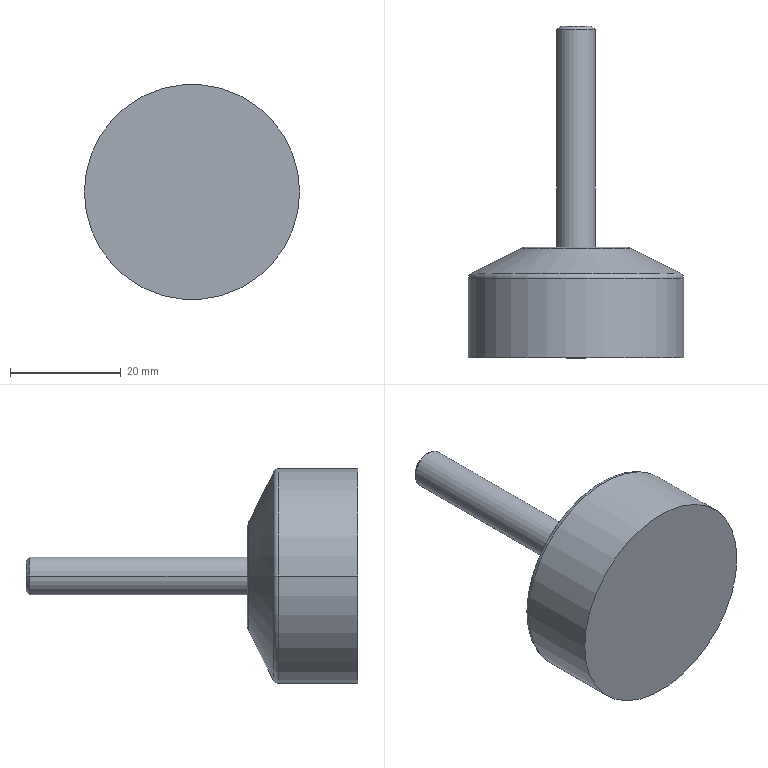Part | SolidWorks | features Revolution 1 | 1 solid | 15 faces | box 38.92 x 60 x 38.92 mm | volume 22752 mm3 | torus 4 | cone 4 | cylinder 4 | plane 3 | commonest cylinder face diameters 6.92 x2 38.92 x2
STEP:
#1=CARTESIAN_POINT('',(-18.92,-10.618,0.));
#2=VERTEX_POINT('',#1);
#3=CARTESIAN_POINT('',(20.,-10.618,0.));
#4=VERTEX_POINT('',#3);
#5=CARTESIAN_POINT('',(0.54,-10.618,0.));
#6=DIRECTION('',(0.,1.,0.));
#7=DIRECTION('',(-1.,0.,0.));
#8=AXIS2_PLACEMENT_3D('',#5,#6,#7);
#9=CIRCLE('',#8,19.46);
#10=EDGE_CURVE('',#2,#4,#9,.T.);
#11=ORIENTED_EDGE('',*,*,#10,.T.);
#12=CARTESIAN_POINT('',(19.447,-9.724,0.));
#13=VERTEX_POINT('',#12);
#14=CARTESIAN_POINT('',(19.,-10.618,0.));
#15=DIRECTION('',(0.,0.,1.));
#16=DIRECTION('',(1.,0.,0.));
#17=AXIS2_PLACEMENT_3D('',#14,#15,#16);
#18=CIRCLE('',#17,1.);
#19=EDGE_CURVE('',#4,#13,#18,.T.);
#20=ORIENTED_EDGE('',*,*,#19,.T.);
#21=CARTESIAN_POINT('',(-18.367,-9.724,0.));
#22=VERTEX_POINT('',#21);
#23=CARTESIAN_POINT('',(0.54,-9.724,0.));
#24=DIRECTION('',(0.,1.,0.));
#25=DIRECTION('',(-1.,0.,0.));
#26=AXIS2_PLACEMENT_3D('',#23,#24,#25);
#27=CIRCLE('',#26,18.907);
#28=EDGE_CURVE('',#22,#13,#27,.T.);
#29=ORIENTED_EDGE('',*,*,#28,.F.);
#30=CARTESIAN_POINT('',(-17.92,-10.618,0.));
#31=DIRECTION('',(0.,0.,-1.));
#32=DIRECTION('',(-1.,0.,0.));
#33=AXIS2_PLACEMENT_3D('',#30,#31,#32);
#34=CIRCLE('',#33,1.);
#35=EDGE_CURVE('',#2,#22,#34,.T.);
#36=ORIENTED_EDGE('',*,*,#35,.F.);
#37=EDGE_LOOP('',(#11,#20,#29,#36));
#38=FACE_OUTER_BOUND('',#37,.T.);
#39=CARTESIAN_POINT('',(0.54,-10.618,0.));
#40=DIRECTION('',(0.,1.,0.));
#41=DIRECTION('',(-1.,0.,0.));
#42=AXIS2_PLACEMENT_3D('',#39,#40,#41);
#43=TOROIDAL_SURFACE('',#42,18.46,1.);
#44=ADVANCED_FACE('',(#38),#43,.T.);
#45=CARTESIAN_POINT('',(-9.448,-5.264,0.));
#46=VERTEX_POINT('',#45);
#47=CARTESIAN_POINT('',(10.528,-5.264,0.));
#48=VERTEX_POINT('',#47);
#49=CARTESIAN_POINT('',(0.54,-5.264,0.));
#50=DIRECTION('',(0.,1.,0.));
#51=DIRECTION('',(-1.,0.,0.));
#52=AXIS2_PLACEMENT_3D('',#49,#50,#51);
#53=CIRCLE('',#52,9.988);
#54=EDGE_CURVE('',#46,#48,#53,.T.);
#55=ORIENTED_EDGE('',*,*,#54,.F.);
#56=CARTESIAN_POINT('',(-9.448,-5.264,0.));
#57=DIRECTION('',(-0.8944,-0.4472,0.));
#58=VECTOR('',#57,1000.);
#59=LINE('',#56,#58);
#60=EDGE_CURVE('',#46,#22,#59,.T.);
#61=ORIENTED_EDGE('',*,*,#60,.T.);
#62=ORIENTED_EDGE('',*,*,#28,.T.);
#63=CARTESIAN_POINT('',(10.528,-5.264,0.));
#64=DIRECTION('',(0.8944,-0.4472,0.));
#65=VECTOR('',#64,1000.);
#66=LINE('',#63,#65);
#67=EDGE_CURVE('',#48,#13,#66,.T.);
#68=ORIENTED_EDGE('',*,*,#67,.F.);
#69=EDGE_LOOP('',(#55,#61,#62,#68));
#70=FACE_OUTER_BOUND('',#69,.T.);
#71=CARTESIAN_POINT('',(0.54,-5.264,0.));
#72=DIRECTION('',(0.,-1.,0.));
#73=DIRECTION('',(1.,0.,0.));
#74=AXIS2_PLACEMENT_3D('',#71,#72,#73);
#75=CONICAL_SURFACE('',#74,9.988,1.107);
#76=ADVANCED_FACE('',(#70),#75,.T.);
#77=ORIENTED_EDGE('',*,*,#54,.T.);
#78=CARTESIAN_POINT('',(9.41,-5.,0.));
#79=VERTEX_POINT('',#78);
#80=CARTESIAN_POINT('',(9.41,-7.5,0.));
#81=DIRECTION('',(0.,0.,1.));
#82=DIRECTION('',(1.,0.,0.));
#83=AXIS2_PLACEMENT_3D('',#80,#81,#82);
#84=CIRCLE('',#83,2.5);
#85=EDGE_CURVE('',#48,#79,#84,.T.);
#86=ORIENTED_EDGE('',*,*,#85,.T.);
#87=CARTESIAN_POINT('',(-8.33,-5.,0.));
#88=VERTEX_POINT('',#87);
#89=CARTESIAN_POINT('',(0.54,-5.,0.));
#90=DIRECTION('',(0.,1.,0.));
#91=DIRECTION('',(-1.,0.,0.));
#92=AXIS2_PLACEMENT_3D('',#89,#90,#91);
#93=CIRCLE('',#92,8.87);
#94=EDGE_CURVE('',#88,#79,#93,.T.);
#95=ORIENTED_EDGE('',*,*,#94,.F.);
#96=CARTESIAN_POINT('',(-8.33,-7.5,0.));
#97=DIRECTION('',(0.,0.,-1.));
#98=DIRECTION('',(-1.,0.,0.));
#99=AXIS2_PLACEMENT_3D('',#96,#97,#98);
#100=CIRCLE('',#99,2.5);
#101=EDGE_CURVE('',#46,#88,#100,.T.);
#102=ORIENTED_EDGE('',*,*,#101,.F.);
#103=EDGE_LOOP('',(#77,#86,#95,#102));
#104=FACE_OUTER_BOUND('',#103,.T.);
#105=CARTESIAN_POINT('',(0.54,-7.5,0.));
#106=DIRECTION('',(0.,1.,0.));
#107=DIRECTION('',(-1.,0.,0.));
#108=AXIS2_PLACEMENT_3D('',#105,#106,#107);
#109=TOROIDAL_SURFACE('',#108,8.87,2.5);
#110=ADVANCED_FACE('',(#104),#109,.T.);
#111=CARTESIAN_POINT('',(-2.92,-5.,0.));
#112=VERTEX_POINT('',#111);
#113=CARTESIAN_POINT('',(4.,-5.,0.));
#114=VERTEX_POINT('',#113);
#115=CARTESIAN_POINT('',(0.54,-5.,0.));
#116=DIRECTION('',(0.,1.,0.));
#117=DIRECTION('',(-1.,0.,0.));
#118=AXIS2_PLACEMENT_3D('',#115,#116,#117);
#119=CIRCLE('',#118,3.46);
#120=EDGE_CURVE('',#112,#114,#119,.T.);
#121=ORIENTED_EDGE('',*,*,#120,.T.);
#122=CARTESIAN_POINT('',(4.,34.387,0.));
#123=VERTEX_POINT('',#122);
#124=CARTESIAN_POINT('',(4.,-25.,0.));
#125=DIRECTION('',(0.,1.,0.));
#126=VECTOR('',#125,1000.);
#127=LINE('',#124,#126);
#128=EDGE_CURVE('',#114,#123,#127,.T.);
#129=ORIENTED_EDGE('',*,*,#128,.T.);
#130=CARTESIAN_POINT('',(-2.92,34.387,0.));
#131=VERTEX_POINT('',#130);
#132=CARTESIAN_POINT('',(0.54,34.387,0.));
#133=DIRECTION('',(0.,1.,0.));
#134=DIRECTION('',(-1.,0.,0.));
#135=AXIS2_PLACEMENT_3D('',#132,#133,#134);
#136=CIRCLE('',#135,3.46);
#137=EDGE_CURVE('',#131,#123,#136,.T.);
#138=ORIENTED_EDGE('',*,*,#137,.F.);
#139=CARTESIAN_POINT('',(-2.92,-25.,0.));
#140=DIRECTION('',(0.,1.,0.));
#141=VECTOR('',#140,1000.);
#142=LINE('',#139,#141);
#143=EDGE_CURVE('',#112,#131,#142,.T.);
#144=ORIENTED_EDGE('',*,*,#143,.F.);
#145=EDGE_LOOP('',(#121,#129,#138,#144));
#146=FACE_OUTER_BOUND('',#145,.T.);
#147=CARTESIAN_POINT('',(0.54,-25.,0.));
#148=DIRECTION('',(0.,1.,0.));
#149=DIRECTION('',(-1.,0.,0.));
#150=AXIS2_PLACEMENT_3D('',#147,#148,#149);
#151=CYLINDRICAL_SURFACE('',#150,3.46);
#152=ADVANCED_FACE('',(#146),#151,.T.);
#153=CARTESIAN_POINT('',(-2.307,35.,0.));
#154=VERTEX_POINT('',#153);
#155=CARTESIAN_POINT('',(3.387,35.,0.));
#156=VERTEX_POINT('',#155);
#157=CARTESIAN_POINT('',(0.54,35.,0.));
#158=DIRECTION('',(0.,1.,0.));
#159=DIRECTION('',(-1.,0.,0.));
#160=AXIS2_PLACEMENT_3D('',#157,#158,#159);
#161=CIRCLE('',#160,2.847);
#162=EDGE_CURVE('',#154,#156,#161,.T.);
#163=ORIENTED_EDGE('',*,*,#162,.F.);
#164=CARTESIAN_POINT('',(-2.307,35.,0.));
#165=DIRECTION('',(-0.7071,-0.7071,0.));
#166=VECTOR('',#165,1000.);
#167=LINE('',#164,#166);
#168=EDGE_CURVE('',#154,#131,#167,.T.);
#169=ORIENTED_EDGE('',*,*,#168,.T.);
#170=ORIENTED_EDGE('',*,*,#137,.T.);
#171=CARTESIAN_POINT('',(3.387,35.,0.));
#172=DIRECTION('',(0.7071,-0.7071,0.));
#173=VECTOR('',#172,1000.);
#174=LINE('',#171,#173);
#175=EDGE_CURVE('',#156,#123,#174,.T.);
#176=ORIENTED_EDGE('',*,*,#175,.F.);
#177=EDGE_LOOP('',(#163,#169,#170,#176));
#178=FACE_OUTER_BOUND('',#177,.T.);
#179=CARTESIAN_POINT('',(0.54,35.,0.));
#180=DIRECTION('',(0.,-1.,0.));
#181=DIRECTION('',(1.,0.,0.));
#182=AXIS2_PLACEMENT_3D('',#179,#180,#181);
#183=CONICAL_SURFACE('',#182,2.847,0.7854);
#184=ADVANCED_FACE('',(#178),#183,.T.);
#185=CARTESIAN_POINT('',(-18.92,-25.,0.));
#186=VERTEX_POINT('',#185);
#187=CARTESIAN_POINT('',(20.,-25.,0.));
#188=VERTEX_POINT('',#187);
#189=CARTESIAN_POINT('',(0.54,-25.,0.));
#190=DIRECTION('',(0.,1.,0.));
#191=DIRECTION('',(-1.,0.,0.));
#192=AXIS2_PLACEMENT_3D('',#189,#190,#191);
#193=CIRCLE('',#192,19.46);
#194=EDGE_CURVE('',#186,#188,#193,.T.);
#195=ORIENTED_EDGE('',*,*,#194,.T.);
#196=CARTESIAN_POINT('',(20.,-25.,0.));
#197=DIRECTION('',(0.,1.,0.));
#198=VECTOR('',#197,1000.);
#199=LINE('',#196,#198);
#200=EDGE_CURVE('',#188,#4,#199,.T.);
#201=ORIENTED_EDGE('',*,*,#200,.T.);
#202=ORIENTED_EDGE('',*,*,#10,.F.);
#203=CARTESIAN_POINT('',(-18.92,-25.,0.));
#204=DIRECTION('',(0.,1.,0.));
#205=VECTOR('',#204,1000.);
#206=LINE('',#203,#205);
#207=EDGE_CURVE('',#186,#2,#206,.T.);
#208=ORIENTED_EDGE('',*,*,#207,.F.);
#209=EDGE_LOOP('',(#195,#201,#202,#208));
#210=FACE_OUTER_BOUND('',#209,.T.);
#211=CARTESIAN_POINT('',(0.54,-25.,0.));
#212=DIRECTION('',(0.,1.,0.));
#213=DIRECTION('',(-1.,0.,0.));
#214=AXIS2_PLACEMENT_3D('',#211,#212,#213);
#215=CYLINDRICAL_SURFACE('',#214,19.46);
#216=ADVANCED_FACE('',(#210),#215,.T.);
#217=ORIENTED_EDGE('',*,*,#200,.F.);
#218=CARTESIAN_POINT('',(0.54,-25.,0.));
#219=DIRECTION('',(0.,1.,0.));
#220=DIRECTION('',(-1.,0.,0.));
#221=AXIS2_PLACEMENT_3D('',#218,#219,#220);
#222=CIRCLE('',#221,19.46);
#223=EDGE_CURVE('',#188,#186,#222,.T.);
#224=ORIENTED_EDGE('',*,*,#223,.T.);
#225=ORIENTED_EDGE('',*,*,#207,.T.);
#226=CARTESIAN_POINT('',(0.54,-10.618,0.));
#227=DIRECTION('',(0.,1.,0.));
#228=DIRECTION('',(-1.,0.,0.));
#229=AXIS2_PLACEMENT_3D('',#226,#227,#228);
#230=CIRCLE('',#229,19.46);
#231=EDGE_CURVE('',#4,#2,#230,.T.);
#232=ORIENTED_EDGE('',*,*,#231,.F.);
#233=EDGE_LOOP('',(#217,#224,#225,#232));
#234=FACE_OUTER_BOUND('',#233,.T.);
#235=CARTESIAN_POINT('',(0.54,-25.,0.));
#236=DIRECTION('',(0.,1.,0.));
#237=DIRECTION('',(-1.,0.,0.));
#238=AXIS2_PLACEMENT_3D('',#235,#236,#237);
#239=CYLINDRICAL_SURFACE('',#238,19.46);
#240=ADVANCED_FACE('',(#234),#239,.T.);
#241=ORIENTED_EDGE('',*,*,#194,.F.);
#242=ORIENTED_EDGE('',*,*,#223,.F.);
#243=EDGE_LOOP('',(#241,#242));
#244=FACE_OUTER_BOUND('',#243,.T.);
#245=CARTESIAN_POINT('',(20.,-25.,0.));
#246=DIRECTION('',(0.,-1.,0.));
#247=DIRECTION('',(1.,0.,0.));
#248=AXIS2_PLACEMENT_3D('',#245,#246,#247);
#249=PLANE('',#248);
#250=ADVANCED_FACE('',(#244),#249,.T.);
#251=CARTESIAN_POINT('',(0.54,35.,0.));
#252=DIRECTION('',(0.,1.,0.));
#253=DIRECTION('',(-1.,0.,0.));
#254=AXIS2_PLACEMENT_3D('',#251,#252,#253);
#255=CIRCLE('',#254,2.847);
#256=EDGE_CURVE('',#156,#154,#255,.T.);
#257=ORIENTED_EDGE('',*,*,#256,.T.);
#258=ORIENTED_EDGE('',*,*,#162,.T.);
#259=EDGE_LOOP('',(#257,#258));
#260=FACE_OUTER_BOUND('',#259,.T.);
#261=CARTESIAN_POINT('',(0.54,35.,0.));
#262=DIRECTION('',(0.,1.,0.));
#263=DIRECTION('',(-1.,0.,0.));
#264=AXIS2_PLACEMENT_3D('',#261,#262,#263);
#265=PLANE('',#264);
#266=ADVANCED_FACE('',(#260),#265,.T.);
#267=ORIENTED_EDGE('',*,*,#168,.F.);
#268=ORIENTED_EDGE('',*,*,#256,.F.);
#269=ORIENTED_EDGE('',*,*,#175,.T.);
#270=CARTESIAN_POINT('',(0.54,34.387,0.));
#271=DIRECTION('',(0.,1.,0.));
#272=DIRECTION('',(-1.,0.,0.));
#273=AXIS2_PLACEMENT_3D('',#270,#271,#272);
#274=CIRCLE('',#273,3.46);
#275=EDGE_CURVE('',#123,#131,#274,.T.);
#276=ORIENTED_EDGE('',*,*,#275,.T.);
#277=EDGE_LOOP('',(#267,#268,#269,#276));
#278=FACE_OUTER_BOUND('',#277,.T.);
#279=CARTESIAN_POINT('',(0.54,35.,0.));
#280=DIRECTION('',(0.,-1.,0.));
#281=DIRECTION('',(1.,0.,0.));
#282=AXIS2_PLACEMENT_3D('',#279,#280,#281);
#283=CONICAL_SURFACE('',#282,2.847,0.7854);
#284=ADVANCED_FACE('',(#278),#283,.T.);
#285=ORIENTED_EDGE('',*,*,#128,.F.);
#286=CARTESIAN_POINT('',(0.54,-5.,0.));
#287=DIRECTION('',(0.,1.,0.));
#288=DIRECTION('',(-1.,0.,0.));
#289=AXIS2_PLACEMENT_3D('',#286,#287,#288);
#290=CIRCLE('',#289,3.46);
#291=EDGE_CURVE('',#114,#112,#290,.T.);
#292=ORIENTED_EDGE('',*,*,#291,.T.);
#293=ORIENTED_EDGE('',*,*,#143,.T.);
#294=ORIENTED_EDGE('',*,*,#275,.F.);
#295=EDGE_LOOP('',(#285,#292,#293,#294));
#296=FACE_OUTER_BOUND('',#295,.T.);
#297=CARTESIAN_POINT('',(0.54,-25.,0.));
#298=DIRECTION('',(0.,1.,0.));
#299=DIRECTION('',(-1.,0.,0.));
#300=AXIS2_PLACEMENT_3D('',#297,#298,#299);
#301=CYLINDRICAL_SURFACE('',#300,3.46);
#302=ADVANCED_FACE('',(#296),#301,.T.);
#303=ORIENTED_EDGE('',*,*,#94,.T.);
#304=CARTESIAN_POINT('',(0.54,-5.,0.));
#305=DIRECTION('',(0.,1.,0.));
#306=DIRECTION('',(-1.,0.,0.));
#307=AXIS2_PLACEMENT_3D('',#304,#305,#306);
#308=CIRCLE('',#307,8.87);
#309=EDGE_CURVE('',#79,#88,#308,.T.);
#310=ORIENTED_EDGE('',*,*,#309,.T.);
#311=EDGE_LOOP('',(#303,#310));
#312=FACE_OUTER_BOUND('',#311,.T.);
#313=ORIENTED_EDGE('',*,*,#120,.F.);
#314=ORIENTED_EDGE('',*,*,#291,.F.);
#315=EDGE_LOOP('',(#313,#314));
#316=FACE_BOUND('',#315,.T.);
#317=CARTESIAN_POINT('',(4.,-5.,0.));
#318=DIRECTION('',(0.,1.,0.));
#319=DIRECTION('',(-1.,0.,0.));
#320=AXIS2_PLACEMENT_3D('',#317,#318,#319);
#321=PLANE('',#320);
#322=ADVANCED_FACE('',(#312,#316),#321,.T.);
#323=ORIENTED_EDGE('',*,*,#85,.F.);
#324=CARTESIAN_POINT('',(0.54,-5.264,0.));
#325=DIRECTION('',(0.,1.,0.));
#326=DIRECTION('',(-1.,0.,0.));
#327=AXIS2_PLACEMENT_3D('',#324,#325,#326);
#328=CIRCLE('',#327,9.988);
#329=EDGE_CURVE('',#48,#46,#328,.T.);
#330=ORIENTED_EDGE('',*,*,#329,.T.);
#331=ORIENTED_EDGE('',*,*,#101,.T.);
#332=ORIENTED_EDGE('',*,*,#309,.F.);
#333=EDGE_LOOP('',(#323,#330,#331,#332));
#334=FACE_OUTER_BOUND('',#333,.T.);
#335=CARTESIAN_POINT('',(0.54,-7.5,0.));
#336=DIRECTION('',(0.,1.,0.));
#337=DIRECTION('',(-1.,0.,0.));
#338=AXIS2_PLACEMENT_3D('',#335,#336,#337);
#339=TOROIDAL_SURFACE('',#338,8.87,2.5);
#340=ADVANCED_FACE('',(#334),#339,.T.);
#341=ORIENTED_EDGE('',*,*,#60,.F.);
#342=ORIENTED_EDGE('',*,*,#329,.F.);
#343=ORIENTED_EDGE('',*,*,#67,.T.);
#344=CARTESIAN_POINT('',(0.54,-9.724,0.));
#345=DIRECTION('',(0.,1.,0.));
#346=DIRECTION('',(-1.,0.,0.));
#347=AXIS2_PLACEMENT_3D('',#344,#345,#346);
#348=CIRCLE('',#347,18.907);
#349=EDGE_CURVE('',#13,#22,#348,.T.);
#350=ORIENTED_EDGE('',*,*,#349,.T.);
#351=EDGE_LOOP('',(#341,#342,#343,#350));
#352=FACE_OUTER_BOUND('',#351,.T.);
#353=CARTESIAN_POINT('',(0.54,-5.264,0.));
#354=DIRECTION('',(0.,-1.,0.));
#355=DIRECTION('',(1.,0.,0.));
#356=AXIS2_PLACEMENT_3D('',#353,#354,#355);
#357=CONICAL_SURFACE('',#356,9.988,1.107);
#358=ADVANCED_FACE('',(#352),#357,.T.);
#359=ORIENTED_EDGE('',*,*,#19,.F.);
#360=ORIENTED_EDGE('',*,*,#231,.T.);
#361=ORIENTED_EDGE('',*,*,#35,.T.);
#362=ORIENTED_EDGE('',*,*,#349,.F.);
#363=EDGE_LOOP('',(#359,#360,#361,#362));
#364=FACE_OUTER_BOUND('',#363,.T.);
#365=CARTESIAN_POINT('',(0.54,-10.618,0.));
#366=DIRECTION('',(0.,1.,0.));
#367=DIRECTION('',(-1.,0.,0.));
#368=AXIS2_PLACEMENT_3D('',#365,#366,#367);
#369=TOROIDAL_SURFACE('',#368,18.46,1.);
#370=ADVANCED_FACE('',(#364),#369,.T.);
#371=CLOSED_SHELL('',(#44,#76,#110,#152,#184,#216,#240,#250,#266,#284,#302,#322,#340,#358,#370));
#372=MANIFOLD_SOLID_BREP('',#371);
#373=CARTESIAN_POINT('',(0.,0.,0.));
#374=DIRECTION('',(0.,0.,1.));
#375=DIRECTION('',(1.,0.,0.));
#376=AXIS2_PLACEMENT_3D('',#373,#374,#375);
#377=(LENGTH_UNIT()NAMED_UNIT(*)SI_UNIT(.MILLI.,.METRE.));
#378=UNCERTAINTY_MEASURE_WITH_UNIT(LENGTH_MEASURE(0.00001),#377,'','');
#379=(NAMED_UNIT(*)PLANE_ANGLE_UNIT()SI_UNIT($,.RADIAN.));
#380=(NAMED_UNIT(*)SI_UNIT($,.STERADIAN.)SOLID_ANGLE_UNIT());
#381=(GEOMETRIC_REPRESENTATION_CONTEXT(3)GLOBAL_UNCERTAINTY_ASSIGNED_CONTEXT((#378))GLOBAL_UNIT_ASSIGNED_CONTEXT((#377,#379,#380))REPRESENTATION_CONTEXT('',''));
#382=ADVANCED_BREP_SHAPE_REPRESENTATION('',(#372,#376),#381);